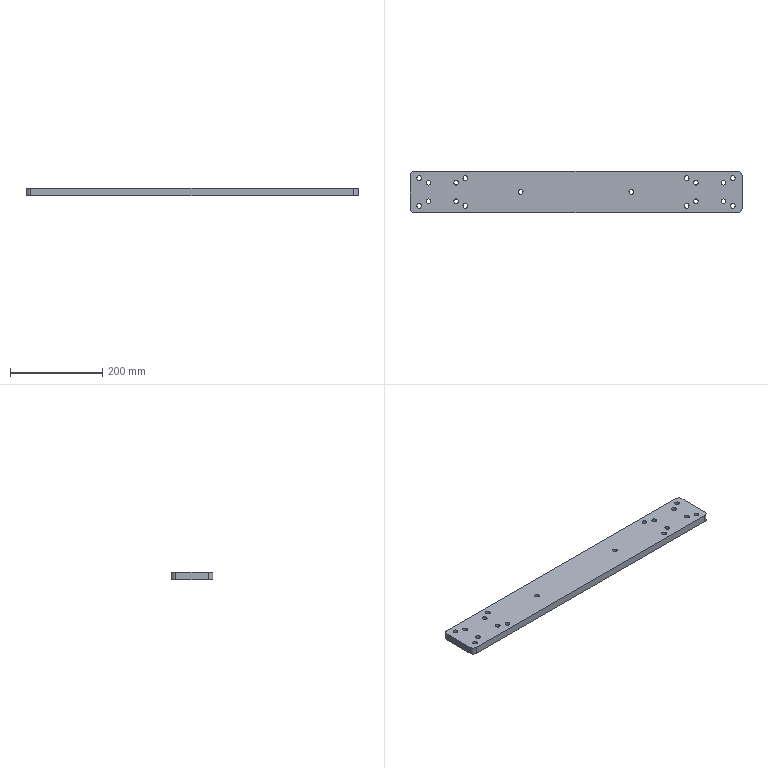Part | STEP file | 1 solid | 46 faces | box 720 x 90 x 16 mm | volume 1011893 mm3 | cylinder 40 | plane 6 | commonest cylinder face diameters 10.2 x36 20 x4